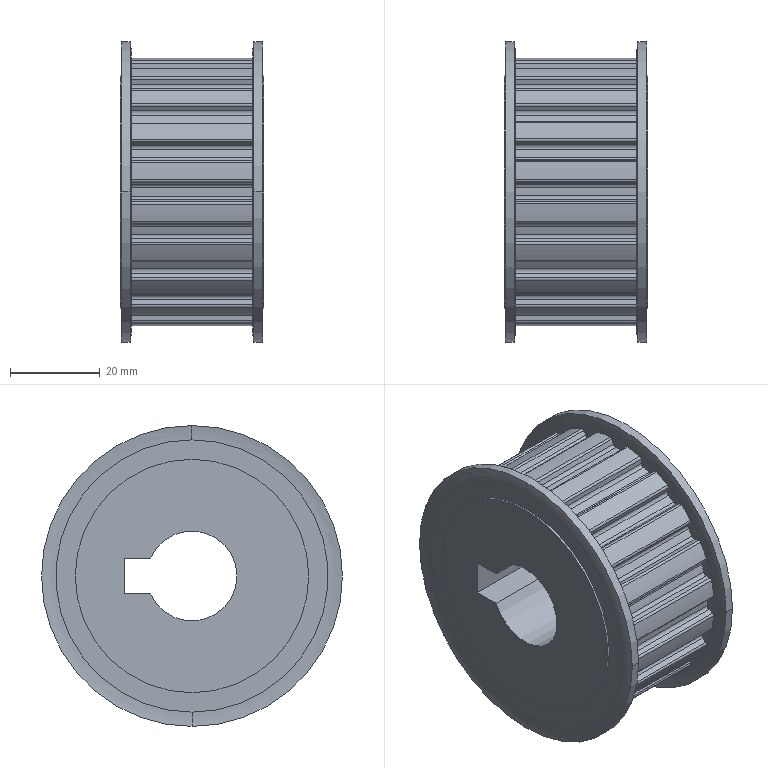Part | SolidWorks | features ICE 1, MBimport 1 | 1 solid | 187 faces | box 32 x 67 x 67 mm | volume 76462 mm3 | cylinder 130 | plane 49 | torus 8 | commonest cylinder face diameters 1.06 x40 1.72 x40 55.62 x20 59.88 x20 52 x4 67 x4